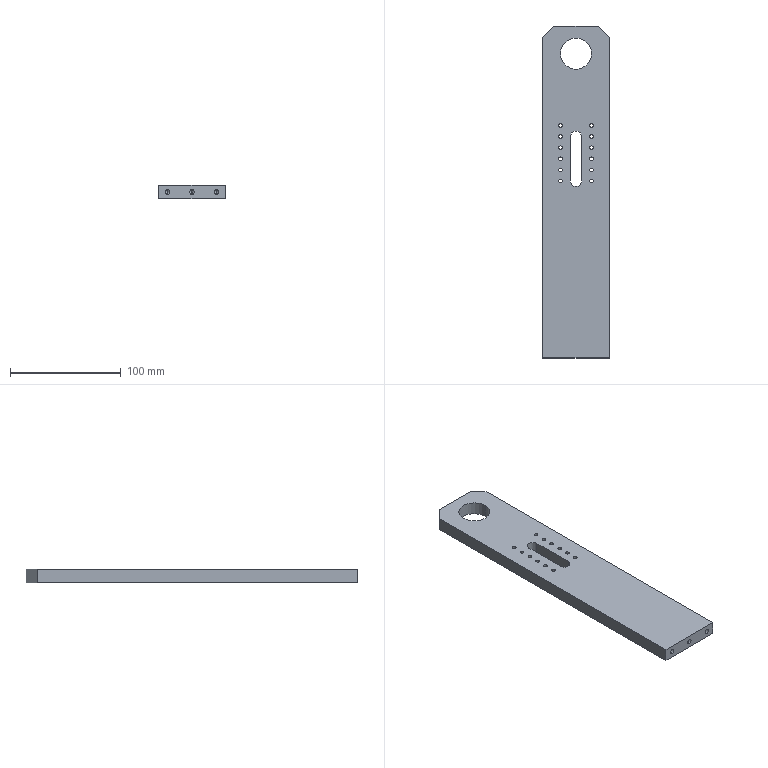Part | STEP file | 11-FG-B06211 | 1 solid | 50 faces | box 60 x 300 x 12 mm | volume 199770 mm3 | cylinder 34 | plane 10 | cone 6 | commonest cylinder face diameters 3.3 x24 4.2 x6 10.2 x2 28 x2